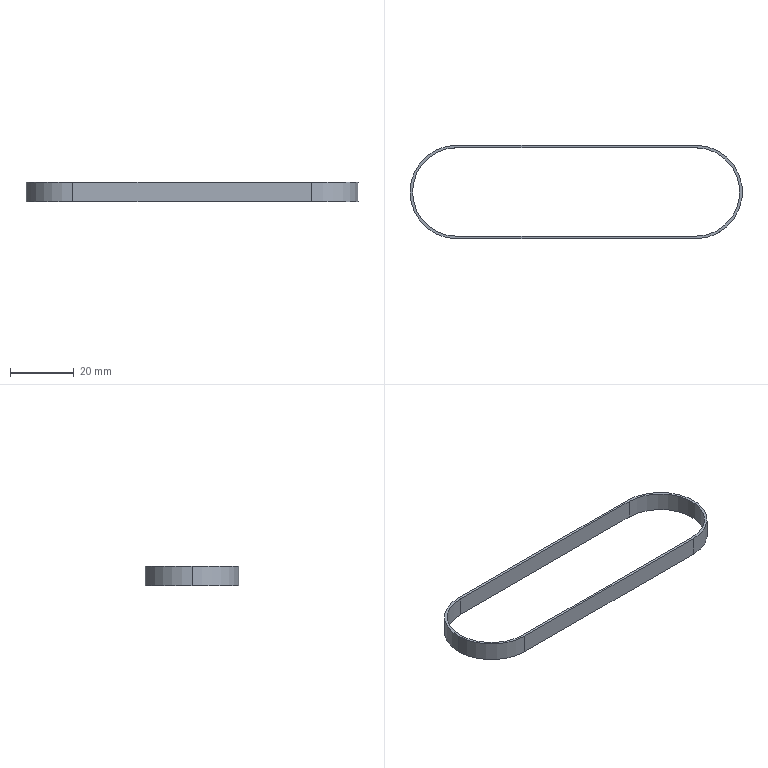Part | STEP file | htun186S3M-60 | 1 solid | 12 faces | box 104.4 x 29.4 x 6 mm | volume 1151 mm3 | cylinder 6 | plane 6 | commonest cylinder face diameters 27.8 x3 29.4 x3
STEP:
#1=CARTESIAN_POINT('',(0.,13.9,6.));
#2=VERTEX_POINT('',#1);
#3=CARTESIAN_POINT('',(-13.9,0.,6.));
#4=VERTEX_POINT('',#3);
#5=CARTESIAN_POINT('',(0.,0.,6.));
#6=DIRECTION('',(0.,0.,1.));
#7=DIRECTION('',(1.,0.,0.));
#8=AXIS2_PLACEMENT_3D('',#5,#6,#7);
#9=CIRCLE('',#8,13.9);
#10=EDGE_CURVE('',#2,#4,#9,.T.);
#11=ORIENTED_EDGE('',*,*,#10,.T.);
#12=CARTESIAN_POINT('',(-13.9,0.,0.));
#13=VERTEX_POINT('',#12);
#14=CARTESIAN_POINT('',(-13.9,0.,6.));
#15=DIRECTION('',(0.,0.,-1.));
#16=VECTOR('',#15,1000.);
#17=LINE('',#14,#16);
#18=EDGE_CURVE('',#4,#13,#17,.T.);
#19=ORIENTED_EDGE('',*,*,#18,.T.);
#20=CARTESIAN_POINT('',(0.,13.9,0.));
#21=VERTEX_POINT('',#20);
#22=CARTESIAN_POINT('',(0.,0.,0.));
#23=DIRECTION('',(0.,0.,1.));
#24=DIRECTION('',(1.,0.,0.));
#25=AXIS2_PLACEMENT_3D('',#22,#23,#24);
#26=CIRCLE('',#25,13.9);
#27=EDGE_CURVE('',#21,#13,#26,.T.);
#28=ORIENTED_EDGE('',*,*,#27,.F.);
#29=CARTESIAN_POINT('',(0.,13.9,6.));
#30=DIRECTION('',(0.,0.,-1.));
#31=VECTOR('',#30,1000.);
#32=LINE('',#29,#31);
#33=EDGE_CURVE('',#2,#21,#32,.T.);
#34=ORIENTED_EDGE('',*,*,#33,.F.);
#35=EDGE_LOOP('',(#11,#19,#28,#34));
#36=FACE_OUTER_BOUND('',#35,.T.);
#37=CARTESIAN_POINT('',(0.,0.,6.));
#38=DIRECTION('',(0.,0.,-1.));
#39=DIRECTION('',(-1.,0.,0.));
#40=AXIS2_PLACEMENT_3D('',#37,#38,#39);
#41=CYLINDRICAL_SURFACE('',#40,13.9);
#42=ADVANCED_FACE('',(#36),#41,.F.);
#43=CARTESIAN_POINT('',(-14.7,0.,6.));
#44=VERTEX_POINT('',#43);
#45=CARTESIAN_POINT('',(0.,-14.7,6.));
#46=VERTEX_POINT('',#45);
#47=CARTESIAN_POINT('',(0.,0.,6.));
#48=DIRECTION('',(0.,0.,1.));
#49=DIRECTION('',(1.,0.,0.));
#50=AXIS2_PLACEMENT_3D('',#47,#48,#49);
#51=CIRCLE('',#50,14.7);
#52=EDGE_CURVE('',#44,#46,#51,.T.);
#53=ORIENTED_EDGE('',*,*,#52,.F.);
#54=CARTESIAN_POINT('',(-14.7,0.,0.));
#55=VERTEX_POINT('',#54);
#56=CARTESIAN_POINT('',(-14.7,0.,6.));
#57=DIRECTION('',(0.,0.,-1.));
#58=VECTOR('',#57,1000.);
#59=LINE('',#56,#58);
#60=EDGE_CURVE('',#44,#55,#59,.T.);
#61=ORIENTED_EDGE('',*,*,#60,.T.);
#62=CARTESIAN_POINT('',(0.,-14.7,0.));
#63=VERTEX_POINT('',#62);
#64=CARTESIAN_POINT('',(0.,0.,0.));
#65=DIRECTION('',(0.,0.,1.));
#66=DIRECTION('',(1.,0.,0.));
#67=AXIS2_PLACEMENT_3D('',#64,#65,#66);
#68=CIRCLE('',#67,14.7);
#69=EDGE_CURVE('',#55,#63,#68,.T.);
#70=ORIENTED_EDGE('',*,*,#69,.T.);
#71=CARTESIAN_POINT('',(0.,-14.7,6.));
#72=DIRECTION('',(0.,0.,-1.));
#73=VECTOR('',#72,1000.);
#74=LINE('',#71,#73);
#75=EDGE_CURVE('',#46,#63,#74,.T.);
#76=ORIENTED_EDGE('',*,*,#75,.F.);
#77=EDGE_LOOP('',(#53,#61,#70,#76));
#78=FACE_OUTER_BOUND('',#77,.T.);
#79=CARTESIAN_POINT('',(0.,0.,6.));
#80=DIRECTION('',(0.,0.,-1.));
#81=DIRECTION('',(-1.,0.,0.));
#82=AXIS2_PLACEMENT_3D('',#79,#80,#81);
#83=CYLINDRICAL_SURFACE('',#82,14.7);
#84=ADVANCED_FACE('',(#78),#83,.T.);
#85=CARTESIAN_POINT('',(0.,14.7,6.));
#86=VERTEX_POINT('',#85);
#87=CARTESIAN_POINT('',(0.,0.,6.));
#88=DIRECTION('',(0.,0.,1.));
#89=DIRECTION('',(1.,0.,0.));
#90=AXIS2_PLACEMENT_3D('',#87,#88,#89);
#91=CIRCLE('',#90,14.7);
#92=EDGE_CURVE('',#86,#44,#91,.T.);
#93=ORIENTED_EDGE('',*,*,#92,.T.);
#94=ORIENTED_EDGE('',*,*,#52,.T.);
#95=CARTESIAN_POINT('',(75.,-14.7,6.));
#96=VERTEX_POINT('',#95);
#97=CARTESIAN_POINT('',(0.,-14.7,6.));
#98=DIRECTION('',(1.,0.,0.));
#99=VECTOR('',#98,1000.);
#100=LINE('',#97,#99);
#101=EDGE_CURVE('',#46,#96,#100,.T.);
#102=ORIENTED_EDGE('',*,*,#101,.T.);
#103=CARTESIAN_POINT('',(75.,14.7,6.));
#104=VERTEX_POINT('',#103);
#105=CARTESIAN_POINT('',(75.,0.,6.));
#106=DIRECTION('',(0.,0.,1.));
#107=DIRECTION('',(1.,0.,0.));
#108=AXIS2_PLACEMENT_3D('',#105,#106,#107);
#109=CIRCLE('',#108,14.7);
#110=EDGE_CURVE('',#96,#104,#109,.T.);
#111=ORIENTED_EDGE('',*,*,#110,.T.);
#112=CARTESIAN_POINT('',(0.,14.7,6.));
#113=DIRECTION('',(-1.,0.,0.));
#114=VECTOR('',#113,1000.);
#115=LINE('',#112,#114);
#116=EDGE_CURVE('',#104,#86,#115,.T.);
#117=ORIENTED_EDGE('',*,*,#116,.T.);
#118=EDGE_LOOP('',(#93,#94,#102,#111,#117));
#119=FACE_OUTER_BOUND('',#118,.T.);
#120=CARTESIAN_POINT('',(0.,-13.9,6.));
#121=VERTEX_POINT('',#120);
#122=CARTESIAN_POINT('',(75.,-13.9,6.));
#123=VERTEX_POINT('',#122);
#124=CARTESIAN_POINT('',(0.,-13.9,6.));
#125=DIRECTION('',(1.,0.,0.));
#126=VECTOR('',#125,1000.);
#127=LINE('',#124,#126);
#128=EDGE_CURVE('',#121,#123,#127,.T.);
#129=ORIENTED_EDGE('',*,*,#128,.F.);
#130=CARTESIAN_POINT('',(0.,0.,6.));
#131=DIRECTION('',(0.,0.,1.));
#132=DIRECTION('',(1.,0.,0.));
#133=AXIS2_PLACEMENT_3D('',#130,#131,#132);
#134=CIRCLE('',#133,13.9);
#135=EDGE_CURVE('',#4,#121,#134,.T.);
#136=ORIENTED_EDGE('',*,*,#135,.F.);
#137=ORIENTED_EDGE('',*,*,#10,.F.);
#138=CARTESIAN_POINT('',(75.,13.9,6.));
#139=VERTEX_POINT('',#138);
#140=CARTESIAN_POINT('',(0.,13.9,6.));
#141=DIRECTION('',(-1.,0.,0.));
#142=VECTOR('',#141,1000.);
#143=LINE('',#140,#142);
#144=EDGE_CURVE('',#139,#2,#143,.T.);
#145=ORIENTED_EDGE('',*,*,#144,.F.);
#146=CARTESIAN_POINT('',(75.,0.,6.));
#147=DIRECTION('',(0.,0.,1.));
#148=DIRECTION('',(1.,0.,0.));
#149=AXIS2_PLACEMENT_3D('',#146,#147,#148);
#150=CIRCLE('',#149,13.9);
#151=EDGE_CURVE('',#123,#139,#150,.T.);
#152=ORIENTED_EDGE('',*,*,#151,.F.);
#153=EDGE_LOOP('',(#129,#136,#137,#145,#152));
#154=FACE_BOUND('',#153,.T.);
#155=CARTESIAN_POINT('',(0.,0.,6.));
#156=DIRECTION('',(0.,0.,1.));
#157=DIRECTION('',(1.,0.,0.));
#158=AXIS2_PLACEMENT_3D('',#155,#156,#157);
#159=PLANE('',#158);
#160=ADVANCED_FACE('',(#119,#154),#159,.T.);
#161=CARTESIAN_POINT('',(0.,14.7,0.));
#162=VERTEX_POINT('',#161);
#163=CARTESIAN_POINT('',(0.,0.,0.));
#164=DIRECTION('',(0.,0.,1.));
#165=DIRECTION('',(1.,0.,0.));
#166=AXIS2_PLACEMENT_3D('',#163,#164,#165);
#167=CIRCLE('',#166,14.7);
#168=EDGE_CURVE('',#162,#55,#167,.T.);
#169=ORIENTED_EDGE('',*,*,#168,.F.);
#170=CARTESIAN_POINT('',(75.,14.7,0.));
#171=VERTEX_POINT('',#170);
#172=CARTESIAN_POINT('',(0.,14.7,0.));
#173=DIRECTION('',(-1.,0.,0.));
#174=VECTOR('',#173,1000.);
#175=LINE('',#172,#174);
#176=EDGE_CURVE('',#171,#162,#175,.T.);
#177=ORIENTED_EDGE('',*,*,#176,.F.);
#178=CARTESIAN_POINT('',(75.,-14.7,0.));
#179=VERTEX_POINT('',#178);
#180=CARTESIAN_POINT('',(75.,0.,0.));
#181=DIRECTION('',(0.,0.,1.));
#182=DIRECTION('',(1.,0.,0.));
#183=AXIS2_PLACEMENT_3D('',#180,#181,#182);
#184=CIRCLE('',#183,14.7);
#185=EDGE_CURVE('',#179,#171,#184,.T.);
#186=ORIENTED_EDGE('',*,*,#185,.F.);
#187=CARTESIAN_POINT('',(0.,-14.7,0.));
#188=DIRECTION('',(1.,0.,0.));
#189=VECTOR('',#188,1000.);
#190=LINE('',#187,#189);
#191=EDGE_CURVE('',#63,#179,#190,.T.);
#192=ORIENTED_EDGE('',*,*,#191,.F.);
#193=ORIENTED_EDGE('',*,*,#69,.F.);
#194=EDGE_LOOP('',(#169,#177,#186,#192,#193));
#195=FACE_OUTER_BOUND('',#194,.T.);
#196=ORIENTED_EDGE('',*,*,#27,.T.);
#197=CARTESIAN_POINT('',(0.,-13.9,0.));
#198=VERTEX_POINT('',#197);
#199=CARTESIAN_POINT('',(0.,0.,0.));
#200=DIRECTION('',(0.,0.,1.));
#201=DIRECTION('',(1.,0.,0.));
#202=AXIS2_PLACEMENT_3D('',#199,#200,#201);
#203=CIRCLE('',#202,13.9);
#204=EDGE_CURVE('',#13,#198,#203,.T.);
#205=ORIENTED_EDGE('',*,*,#204,.T.);
#206=CARTESIAN_POINT('',(75.,-13.9,0.));
#207=VERTEX_POINT('',#206);
#208=CARTESIAN_POINT('',(0.,-13.9,0.));
#209=DIRECTION('',(1.,0.,0.));
#210=VECTOR('',#209,1000.);
#211=LINE('',#208,#210);
#212=EDGE_CURVE('',#198,#207,#211,.T.);
#213=ORIENTED_EDGE('',*,*,#212,.T.);
#214=CARTESIAN_POINT('',(75.,13.9,0.));
#215=VERTEX_POINT('',#214);
#216=CARTESIAN_POINT('',(75.,0.,0.));
#217=DIRECTION('',(0.,0.,1.));
#218=DIRECTION('',(1.,0.,0.));
#219=AXIS2_PLACEMENT_3D('',#216,#217,#218);
#220=CIRCLE('',#219,13.9);
#221=EDGE_CURVE('',#207,#215,#220,.T.);
#222=ORIENTED_EDGE('',*,*,#221,.T.);
#223=CARTESIAN_POINT('',(0.,13.9,0.));
#224=DIRECTION('',(-1.,0.,0.));
#225=VECTOR('',#224,1000.);
#226=LINE('',#223,#225);
#227=EDGE_CURVE('',#215,#21,#226,.T.);
#228=ORIENTED_EDGE('',*,*,#227,.T.);
#229=EDGE_LOOP('',(#196,#205,#213,#222,#228));
#230=FACE_BOUND('',#229,.T.);
#231=CARTESIAN_POINT('',(0.,0.,0.));
#232=DIRECTION('',(0.,0.,1.));
#233=DIRECTION('',(1.,0.,0.));
#234=AXIS2_PLACEMENT_3D('',#231,#232,#233);
#235=PLANE('',#234);
#236=ADVANCED_FACE('',(#195,#230),#235,.F.);
#237=ORIENTED_EDGE('',*,*,#60,.F.);
#238=ORIENTED_EDGE('',*,*,#92,.F.);
#239=CARTESIAN_POINT('',(0.,14.7,6.));
#240=DIRECTION('',(0.,0.,-1.));
#241=VECTOR('',#240,1000.);
#242=LINE('',#239,#241);
#243=EDGE_CURVE('',#86,#162,#242,.T.);
#244=ORIENTED_EDGE('',*,*,#243,.T.);
#245=ORIENTED_EDGE('',*,*,#168,.T.);
#246=EDGE_LOOP('',(#237,#238,#244,#245));
#247=FACE_OUTER_BOUND('',#246,.T.);
#248=CARTESIAN_POINT('',(0.,0.,6.));
#249=DIRECTION('',(0.,0.,-1.));
#250=DIRECTION('',(-1.,0.,0.));
#251=AXIS2_PLACEMENT_3D('',#248,#249,#250);
#252=CYLINDRICAL_SURFACE('',#251,14.7);
#253=ADVANCED_FACE('',(#247),#252,.T.);
#254=ORIENTED_EDGE('',*,*,#191,.T.);
#255=CARTESIAN_POINT('',(75.,-14.7,6.));
#256=DIRECTION('',(0.,0.,-1.));
#257=VECTOR('',#256,1000.);
#258=LINE('',#255,#257);
#259=EDGE_CURVE('',#96,#179,#258,.T.);
#260=ORIENTED_EDGE('',*,*,#259,.F.);
#261=ORIENTED_EDGE('',*,*,#101,.F.);
#262=ORIENTED_EDGE('',*,*,#75,.T.);
#263=EDGE_LOOP('',(#254,#260,#261,#262));
#264=FACE_OUTER_BOUND('',#263,.T.);
#265=CARTESIAN_POINT('',(0.,-14.7,6.));
#266=DIRECTION('',(0.,1.,0.));
#267=DIRECTION('',(-1.,0.,0.));
#268=AXIS2_PLACEMENT_3D('',#265,#266,#267);
#269=PLANE('',#268);
#270=ADVANCED_FACE('',(#264),#269,.F.);
#271=ORIENTED_EDGE('',*,*,#185,.T.);
#272=CARTESIAN_POINT('',(75.,14.7,6.));
#273=DIRECTION('',(0.,0.,-1.));
#274=VECTOR('',#273,1000.);
#275=LINE('',#272,#274);
#276=EDGE_CURVE('',#104,#171,#275,.T.);
#277=ORIENTED_EDGE('',*,*,#276,.F.);
#278=ORIENTED_EDGE('',*,*,#110,.F.);
#279=ORIENTED_EDGE('',*,*,#259,.T.);
#280=EDGE_LOOP('',(#271,#277,#278,#279));
#281=FACE_OUTER_BOUND('',#280,.T.);
#282=CARTESIAN_POINT('',(75.,0.,6.));
#283=DIRECTION('',(0.,0.,-1.));
#284=DIRECTION('',(-1.,0.,0.));
#285=AXIS2_PLACEMENT_3D('',#282,#283,#284);
#286=CYLINDRICAL_SURFACE('',#285,14.7);
#287=ADVANCED_FACE('',(#281),#286,.T.);
#288=ORIENTED_EDGE('',*,*,#176,.T.);
#289=ORIENTED_EDGE('',*,*,#243,.F.);
#290=ORIENTED_EDGE('',*,*,#116,.F.);
#291=ORIENTED_EDGE('',*,*,#276,.T.);
#292=EDGE_LOOP('',(#288,#289,#290,#291));
#293=FACE_OUTER_BOUND('',#292,.T.);
#294=CARTESIAN_POINT('',(0.,14.7,6.));
#295=DIRECTION('',(0.,-1.,0.));
#296=DIRECTION('',(0.,0.,-1.));
#297=AXIS2_PLACEMENT_3D('',#294,#295,#296);
#298=PLANE('',#297);
#299=ADVANCED_FACE('',(#293),#298,.F.);
#300=ORIENTED_EDGE('',*,*,#18,.F.);
#301=ORIENTED_EDGE('',*,*,#135,.T.);
#302=CARTESIAN_POINT('',(0.,-13.9,6.));
#303=DIRECTION('',(0.,0.,-1.));
#304=VECTOR('',#303,1000.);
#305=LINE('',#302,#304);
#306=EDGE_CURVE('',#121,#198,#305,.T.);
#307=ORIENTED_EDGE('',*,*,#306,.T.);
#308=ORIENTED_EDGE('',*,*,#204,.F.);
#309=EDGE_LOOP('',(#300,#301,#307,#308));
#310=FACE_OUTER_BOUND('',#309,.T.);
#311=CARTESIAN_POINT('',(0.,0.,6.));
#312=DIRECTION('',(0.,0.,-1.));
#313=DIRECTION('',(-1.,0.,0.));
#314=AXIS2_PLACEMENT_3D('',#311,#312,#313);
#315=CYLINDRICAL_SURFACE('',#314,13.9);
#316=ADVANCED_FACE('',(#310),#315,.F.);
#317=ORIENTED_EDGE('',*,*,#212,.F.);
#318=ORIENTED_EDGE('',*,*,#306,.F.);
#319=ORIENTED_EDGE('',*,*,#128,.T.);
#320=CARTESIAN_POINT('',(75.,-13.9,6.));
#321=DIRECTION('',(0.,0.,-1.));
#322=VECTOR('',#321,1000.);
#323=LINE('',#320,#322);
#324=EDGE_CURVE('',#123,#207,#323,.T.);
#325=ORIENTED_EDGE('',*,*,#324,.T.);
#326=EDGE_LOOP('',(#317,#318,#319,#325));
#327=FACE_OUTER_BOUND('',#326,.T.);
#328=CARTESIAN_POINT('',(0.,-13.9,6.));
#329=DIRECTION('',(0.,1.,0.));
#330=DIRECTION('',(-1.,0.,0.));
#331=AXIS2_PLACEMENT_3D('',#328,#329,#330);
#332=PLANE('',#331);
#333=ADVANCED_FACE('',(#327),#332,.T.);
#334=ORIENTED_EDGE('',*,*,#221,.F.);
#335=ORIENTED_EDGE('',*,*,#324,.F.);
#336=ORIENTED_EDGE('',*,*,#151,.T.);
#337=CARTESIAN_POINT('',(75.,13.9,6.));
#338=DIRECTION('',(0.,0.,-1.));
#339=VECTOR('',#338,1000.);
#340=LINE('',#337,#339);
#341=EDGE_CURVE('',#139,#215,#340,.T.);
#342=ORIENTED_EDGE('',*,*,#341,.T.);
#343=EDGE_LOOP('',(#334,#335,#336,#342));
#344=FACE_OUTER_BOUND('',#343,.T.);
#345=CARTESIAN_POINT('',(75.,0.,6.));
#346=DIRECTION('',(0.,0.,-1.));
#347=DIRECTION('',(-1.,0.,0.));
#348=AXIS2_PLACEMENT_3D('',#345,#346,#347);
#349=CYLINDRICAL_SURFACE('',#348,13.9);
#350=ADVANCED_FACE('',(#344),#349,.F.);
#351=ORIENTED_EDGE('',*,*,#227,.F.);
#352=ORIENTED_EDGE('',*,*,#341,.F.);
#353=ORIENTED_EDGE('',*,*,#144,.T.);
#354=ORIENTED_EDGE('',*,*,#33,.T.);
#355=EDGE_LOOP('',(#351,#352,#353,#354));
#356=FACE_OUTER_BOUND('',#355,.T.);
#357=CARTESIAN_POINT('',(0.,13.9,6.));
#358=DIRECTION('',(0.,-1.,0.));
#359=DIRECTION('',(1.,0.,0.));
#360=AXIS2_PLACEMENT_3D('',#357,#358,#359);
#361=PLANE('',#360);
#362=ADVANCED_FACE('',(#356),#361,.T.);
#363=CLOSED_SHELL('',(#42,#84,#160,#236,#253,#270,#287,#299,#316,#333,#350,#362));
#364=MANIFOLD_SOLID_BREP('',#363);
#365=CARTESIAN_POINT('',(0.,0.,0.));
#366=DIRECTION('',(0.,0.,1.));
#367=DIRECTION('',(1.,0.,0.));
#368=AXIS2_PLACEMENT_3D('',#365,#366,#367);
#369=(LENGTH_UNIT()NAMED_UNIT(*)SI_UNIT(.MILLI.,.METRE.));
#370=UNCERTAINTY_MEASURE_WITH_UNIT(LENGTH_MEASURE(0.00001),#369,'','');
#371=(NAMED_UNIT(*)PLANE_ANGLE_UNIT()SI_UNIT($,.RADIAN.));
#372=(NAMED_UNIT(*)SI_UNIT($,.STERADIAN.)SOLID_ANGLE_UNIT());
#373=(GEOMETRIC_REPRESENTATION_CONTEXT(3)GLOBAL_UNCERTAINTY_ASSIGNED_CONTEXT((#370))GLOBAL_UNIT_ASSIGNED_CONTEXT((#369,#371,#372))REPRESENTATION_CONTEXT('',''));
#374=ADVANCED_BREP_SHAPE_REPRESENTATION('',(#364,#368),#373);